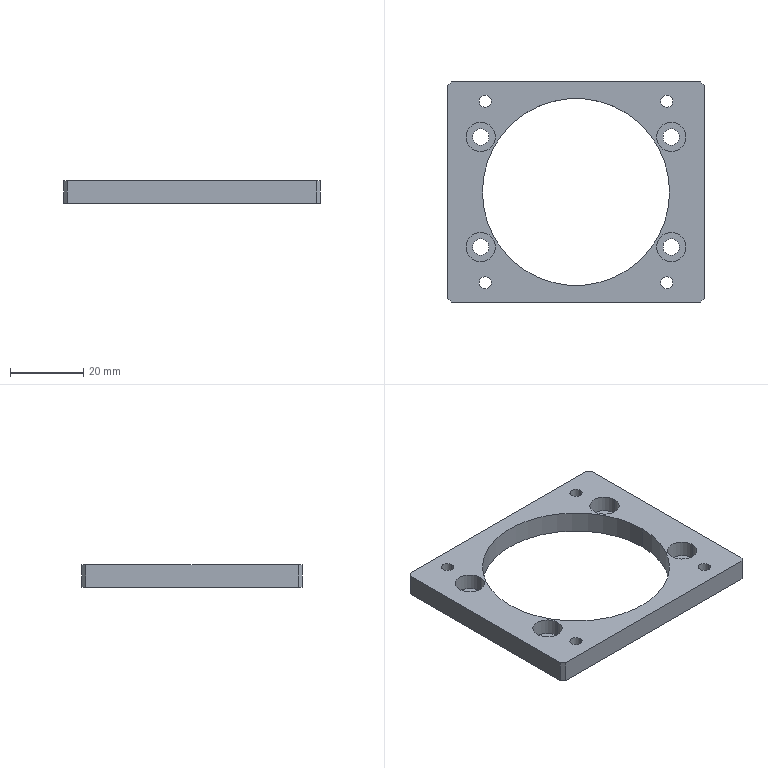Part | NX | features BREP 1 | 1 solid | 40 faces | box 70 x 60 x 6 mm | volume 11726 mm3 | cylinder 26 | plane 14 | commonest cylinder face diameters 3.3 x8 4.5 x8 8 x8 51 x2
STEP:
#1=CARTESIAN_POINT('',(58.099,54.749,0.));
#2=VERTEX_POINT('',#1);
#3=CARTESIAN_POINT('',(61.399,54.749,0.));
#4=VERTEX_POINT('',#3);
#5=CARTESIAN_POINT('',(59.749,54.749,0.));
#6=DIRECTION('',(0.,0.,1.));
#7=DIRECTION('',(1.,0.,0.));
#8=AXIS2_PLACEMENT_3D('',#5,#6,#7);
#9=CIRCLE('',#8,1.65);
#10=EDGE_CURVE('',#2,#4,#9,.T.);
#11=ORIENTED_EDGE('',*,*,#10,.F.);
#12=CARTESIAN_POINT('',(58.099,54.749,6.));
#13=VERTEX_POINT('',#12);
#14=CARTESIAN_POINT('',(58.099,54.749,6.));
#15=DIRECTION('',(0.,0.,1.));
#16=VECTOR('',#15,1000.);
#17=LINE('',#14,#16);
#18=EDGE_CURVE('',#13,#2,#17,.F.);
#19=ORIENTED_EDGE('',*,*,#18,.F.);
#20=CARTESIAN_POINT('',(61.399,54.749,6.));
#21=VERTEX_POINT('',#20);
#22=CARTESIAN_POINT('',(59.749,54.749,6.));
#23=DIRECTION('',(0.,0.,1.));
#24=DIRECTION('',(1.,0.,0.));
#25=AXIS2_PLACEMENT_3D('',#22,#23,#24);
#26=CIRCLE('',#25,1.65);
#27=EDGE_CURVE('',#13,#21,#26,.T.);
#28=ORIENTED_EDGE('',*,*,#27,.T.);
#29=CARTESIAN_POINT('',(61.399,54.749,6.));
#30=DIRECTION('',(0.,0.,1.));
#31=VECTOR('',#30,1000.);
#32=LINE('',#29,#31);
#33=EDGE_CURVE('',#21,#4,#32,.F.);
#34=ORIENTED_EDGE('',*,*,#33,.T.);
#35=EDGE_LOOP('',(#11,#19,#28,#34));
#36=FACE_BOUND('',#35,.T.);
#37=CARTESIAN_POINT('',(59.749,54.749,6.));
#38=DIRECTION('',(0.,0.,1.));
#39=DIRECTION('',(1.,0.,0.));
#40=AXIS2_PLACEMENT_3D('',#37,#38,#39);
#41=CYLINDRICAL_SURFACE('',#40,1.65);
#42=ADVANCED_FACE('',(#36),#41,.F.);
#43=CARTESIAN_POINT('',(58.099,5.251,0.));
#44=VERTEX_POINT('',#43);
#45=CARTESIAN_POINT('',(61.399,5.251,0.));
#46=VERTEX_POINT('',#45);
#47=CARTESIAN_POINT('',(59.749,5.251,0.));
#48=DIRECTION('',(0.,0.,1.));
#49=DIRECTION('',(1.,0.,0.));
#50=AXIS2_PLACEMENT_3D('',#47,#48,#49);
#51=CIRCLE('',#50,1.65);
#52=EDGE_CURVE('',#44,#46,#51,.T.);
#53=ORIENTED_EDGE('',*,*,#52,.F.);
#54=CARTESIAN_POINT('',(58.099,5.251,6.));
#55=VERTEX_POINT('',#54);
#56=CARTESIAN_POINT('',(58.099,5.251,6.));
#57=DIRECTION('',(0.,0.,1.));
#58=VECTOR('',#57,1000.);
#59=LINE('',#56,#58);
#60=EDGE_CURVE('',#55,#44,#59,.F.);
#61=ORIENTED_EDGE('',*,*,#60,.F.);
#62=CARTESIAN_POINT('',(61.399,5.251,6.));
#63=VERTEX_POINT('',#62);
#64=CARTESIAN_POINT('',(59.749,5.251,6.));
#65=DIRECTION('',(0.,0.,1.));
#66=DIRECTION('',(1.,0.,0.));
#67=AXIS2_PLACEMENT_3D('',#64,#65,#66);
#68=CIRCLE('',#67,1.65);
#69=EDGE_CURVE('',#55,#63,#68,.T.);
#70=ORIENTED_EDGE('',*,*,#69,.T.);
#71=CARTESIAN_POINT('',(61.399,5.251,6.));
#72=DIRECTION('',(0.,0.,1.));
#73=VECTOR('',#72,1000.);
#74=LINE('',#71,#73);
#75=EDGE_CURVE('',#63,#46,#74,.F.);
#76=ORIENTED_EDGE('',*,*,#75,.T.);
#77=EDGE_LOOP('',(#53,#61,#70,#76));
#78=FACE_BOUND('',#77,.T.);
#79=CARTESIAN_POINT('',(59.749,5.251,6.));
#80=DIRECTION('',(0.,0.,1.));
#81=DIRECTION('',(1.,0.,0.));
#82=AXIS2_PLACEMENT_3D('',#79,#80,#81);
#83=CYLINDRICAL_SURFACE('',#82,1.65);
#84=ADVANCED_FACE('',(#78),#83,.F.);
#85=CARTESIAN_POINT('',(8.601,5.251,0.));
#86=VERTEX_POINT('',#85);
#87=CARTESIAN_POINT('',(11.901,5.251,0.));
#88=VERTEX_POINT('',#87);
#89=CARTESIAN_POINT('',(10.251,5.251,0.));
#90=DIRECTION('',(0.,0.,1.));
#91=DIRECTION('',(1.,0.,0.));
#92=AXIS2_PLACEMENT_3D('',#89,#90,#91);
#93=CIRCLE('',#92,1.65);
#94=EDGE_CURVE('',#86,#88,#93,.T.);
#95=ORIENTED_EDGE('',*,*,#94,.F.);
#96=CARTESIAN_POINT('',(8.601,5.251,6.));
#97=VERTEX_POINT('',#96);
#98=CARTESIAN_POINT('',(8.601,5.251,6.));
#99=DIRECTION('',(0.,0.,1.));
#100=VECTOR('',#99,1000.);
#101=LINE('',#98,#100);
#102=EDGE_CURVE('',#97,#86,#101,.F.);
#103=ORIENTED_EDGE('',*,*,#102,.F.);
#104=CARTESIAN_POINT('',(11.901,5.251,6.));
#105=VERTEX_POINT('',#104);
#106=CARTESIAN_POINT('',(10.251,5.251,6.));
#107=DIRECTION('',(0.,0.,1.));
#108=DIRECTION('',(1.,0.,0.));
#109=AXIS2_PLACEMENT_3D('',#106,#107,#108);
#110=CIRCLE('',#109,1.65);
#111=EDGE_CURVE('',#97,#105,#110,.T.);
#112=ORIENTED_EDGE('',*,*,#111,.T.);
#113=CARTESIAN_POINT('',(11.901,5.251,6.));
#114=DIRECTION('',(0.,0.,1.));
#115=VECTOR('',#114,1000.);
#116=LINE('',#113,#115);
#117=EDGE_CURVE('',#105,#88,#116,.F.);
#118=ORIENTED_EDGE('',*,*,#117,.T.);
#119=EDGE_LOOP('',(#95,#103,#112,#118));
#120=FACE_BOUND('',#119,.T.);
#121=CARTESIAN_POINT('',(10.251,5.251,6.));
#122=DIRECTION('',(0.,0.,1.));
#123=DIRECTION('',(1.,0.,0.));
#124=AXIS2_PLACEMENT_3D('',#121,#122,#123);
#125=CYLINDRICAL_SURFACE('',#124,1.65);
#126=ADVANCED_FACE('',(#120),#125,.F.);
#127=CARTESIAN_POINT('',(8.601,54.749,0.));
#128=VERTEX_POINT('',#127);
#129=CARTESIAN_POINT('',(11.901,54.749,0.));
#130=VERTEX_POINT('',#129);
#131=CARTESIAN_POINT('',(10.251,54.749,0.));
#132=DIRECTION('',(0.,0.,1.));
#133=DIRECTION('',(1.,0.,0.));
#134=AXIS2_PLACEMENT_3D('',#131,#132,#133);
#135=CIRCLE('',#134,1.65);
#136=EDGE_CURVE('',#128,#130,#135,.T.);
#137=ORIENTED_EDGE('',*,*,#136,.F.);
#138=CARTESIAN_POINT('',(8.601,54.749,6.));
#139=VERTEX_POINT('',#138);
#140=CARTESIAN_POINT('',(8.601,54.749,6.));
#141=DIRECTION('',(0.,0.,1.));
#142=VECTOR('',#141,1000.);
#143=LINE('',#140,#142);
#144=EDGE_CURVE('',#139,#128,#143,.F.);
#145=ORIENTED_EDGE('',*,*,#144,.F.);
#146=CARTESIAN_POINT('',(11.901,54.749,6.));
#147=VERTEX_POINT('',#146);
#148=CARTESIAN_POINT('',(10.251,54.749,6.));
#149=DIRECTION('',(0.,0.,1.));
#150=DIRECTION('',(1.,0.,0.));
#151=AXIS2_PLACEMENT_3D('',#148,#149,#150);
#152=CIRCLE('',#151,1.65);
#153=EDGE_CURVE('',#139,#147,#152,.T.);
#154=ORIENTED_EDGE('',*,*,#153,.T.);
#155=CARTESIAN_POINT('',(11.901,54.749,6.));
#156=DIRECTION('',(0.,0.,1.));
#157=VECTOR('',#156,1000.);
#158=LINE('',#155,#157);
#159=EDGE_CURVE('',#147,#130,#158,.F.);
#160=ORIENTED_EDGE('',*,*,#159,.T.);
#161=EDGE_LOOP('',(#137,#145,#154,#160));
#162=FACE_BOUND('',#161,.T.);
#163=CARTESIAN_POINT('',(10.251,54.749,6.));
#164=DIRECTION('',(0.,0.,1.));
#165=DIRECTION('',(1.,0.,0.));
#166=AXIS2_PLACEMENT_3D('',#163,#164,#165);
#167=CYLINDRICAL_SURFACE('',#166,1.65);
#168=ADVANCED_FACE('',(#162),#167,.F.);
#169=CARTESIAN_POINT('',(56.981,45.,1.5));
#170=VERTEX_POINT('',#169);
#171=CARTESIAN_POINT('',(64.981,45.,1.5));
#172=VERTEX_POINT('',#171);
#173=CARTESIAN_POINT('',(60.981,45.,1.5));
#174=DIRECTION('',(0.,0.,1.));
#175=DIRECTION('',(1.,0.,0.));
#176=AXIS2_PLACEMENT_3D('',#173,#174,#175);
#177=CIRCLE('',#176,4.);
#178=EDGE_CURVE('',#170,#172,#177,.T.);
#179=ORIENTED_EDGE('',*,*,#178,.F.);
#180=CARTESIAN_POINT('',(56.981,45.,6.));
#181=VERTEX_POINT('',#180);
#182=CARTESIAN_POINT('',(56.981,45.,6.));
#183=DIRECTION('',(0.,0.,1.));
#184=VECTOR('',#183,1000.);
#185=LINE('',#182,#184);
#186=EDGE_CURVE('',#181,#170,#185,.F.);
#187=ORIENTED_EDGE('',*,*,#186,.F.);
#188=CARTESIAN_POINT('',(64.981,45.,6.));
#189=VERTEX_POINT('',#188);
#190=CARTESIAN_POINT('',(60.981,45.,6.));
#191=DIRECTION('',(0.,0.,1.));
#192=DIRECTION('',(1.,0.,0.));
#193=AXIS2_PLACEMENT_3D('',#190,#191,#192);
#194=CIRCLE('',#193,4.);
#195=EDGE_CURVE('',#181,#189,#194,.T.);
#196=ORIENTED_EDGE('',*,*,#195,.T.);
#197=CARTESIAN_POINT('',(64.981,45.,6.));
#198=DIRECTION('',(0.,0.,1.));
#199=VECTOR('',#198,1000.);
#200=LINE('',#197,#199);
#201=EDGE_CURVE('',#189,#172,#200,.F.);
#202=ORIENTED_EDGE('',*,*,#201,.T.);
#203=EDGE_LOOP('',(#179,#187,#196,#202));
#204=FACE_BOUND('',#203,.T.);
#205=CARTESIAN_POINT('',(60.981,45.,6.));
#206=DIRECTION('',(0.,0.,1.));
#207=DIRECTION('',(1.,0.,0.));
#208=AXIS2_PLACEMENT_3D('',#205,#206,#207);
#209=CYLINDRICAL_SURFACE('',#208,4.);
#210=ADVANCED_FACE('',(#204),#209,.F.);
#211=CARTESIAN_POINT('',(58.731,45.,0.));
#212=VERTEX_POINT('',#211);
#213=CARTESIAN_POINT('',(63.231,45.,0.));
#214=VERTEX_POINT('',#213);
#215=CARTESIAN_POINT('',(60.981,45.,0.));
#216=DIRECTION('',(0.,0.,1.));
#217=DIRECTION('',(1.,0.,0.));
#218=AXIS2_PLACEMENT_3D('',#215,#216,#217);
#219=CIRCLE('',#218,2.25);
#220=EDGE_CURVE('',#212,#214,#219,.T.);
#221=ORIENTED_EDGE('',*,*,#220,.F.);
#222=CARTESIAN_POINT('',(58.731,45.,1.5));
#223=VERTEX_POINT('',#222);
#224=CARTESIAN_POINT('',(58.731,45.,6.));
#225=DIRECTION('',(0.,0.,1.));
#226=VECTOR('',#225,1000.);
#227=LINE('',#224,#226);
#228=EDGE_CURVE('',#223,#212,#227,.F.);
#229=ORIENTED_EDGE('',*,*,#228,.F.);
#230=CARTESIAN_POINT('',(63.231,45.,1.5));
#231=VERTEX_POINT('',#230);
#232=CARTESIAN_POINT('',(60.981,45.,1.5));
#233=DIRECTION('',(0.,0.,1.));
#234=DIRECTION('',(1.,0.,0.));
#235=AXIS2_PLACEMENT_3D('',#232,#233,#234);
#236=CIRCLE('',#235,2.25);
#237=EDGE_CURVE('',#223,#231,#236,.T.);
#238=ORIENTED_EDGE('',*,*,#237,.T.);
#239=CARTESIAN_POINT('',(63.231,45.,6.));
#240=DIRECTION('',(0.,0.,1.));
#241=VECTOR('',#240,1000.);
#242=LINE('',#239,#241);
#243=EDGE_CURVE('',#231,#214,#242,.F.);
#244=ORIENTED_EDGE('',*,*,#243,.T.);
#245=EDGE_LOOP('',(#221,#229,#238,#244));
#246=FACE_BOUND('',#245,.T.);
#247=CARTESIAN_POINT('',(60.981,45.,6.));
#248=DIRECTION('',(0.,0.,1.));
#249=DIRECTION('',(1.,0.,0.));
#250=AXIS2_PLACEMENT_3D('',#247,#248,#249);
#251=CYLINDRICAL_SURFACE('',#250,2.25);
#252=ADVANCED_FACE('',(#246),#251,.F.);
#253=CARTESIAN_POINT('',(5.019,15.,1.5));
#254=VERTEX_POINT('',#253);
#255=CARTESIAN_POINT('',(13.019,15.,1.5));
#256=VERTEX_POINT('',#255);
#257=CARTESIAN_POINT('',(9.019,15.,1.5));
#258=DIRECTION('',(0.,0.,1.));
#259=DIRECTION('',(1.,0.,0.));
#260=AXIS2_PLACEMENT_3D('',#257,#258,#259);
#261=CIRCLE('',#260,4.);
#262=EDGE_CURVE('',#254,#256,#261,.T.);
#263=ORIENTED_EDGE('',*,*,#262,.F.);
#264=CARTESIAN_POINT('',(5.019,15.,6.));
#265=VERTEX_POINT('',#264);
#266=CARTESIAN_POINT('',(5.019,15.,6.));
#267=DIRECTION('',(0.,0.,1.));
#268=VECTOR('',#267,1000.);
#269=LINE('',#266,#268);
#270=EDGE_CURVE('',#265,#254,#269,.F.);
#271=ORIENTED_EDGE('',*,*,#270,.F.);
#272=CARTESIAN_POINT('',(13.019,15.,6.));
#273=VERTEX_POINT('',#272);
#274=CARTESIAN_POINT('',(9.019,15.,6.));
#275=DIRECTION('',(0.,0.,1.));
#276=DIRECTION('',(1.,0.,0.));
#277=AXIS2_PLACEMENT_3D('',#274,#275,#276);
#278=CIRCLE('',#277,4.);
#279=EDGE_CURVE('',#265,#273,#278,.T.);
#280=ORIENTED_EDGE('',*,*,#279,.T.);
#281=CARTESIAN_POINT('',(13.019,15.,6.));
#282=DIRECTION('',(0.,0.,1.));
#283=VECTOR('',#282,1000.);
#284=LINE('',#281,#283);
#285=EDGE_CURVE('',#273,#256,#284,.F.);
#286=ORIENTED_EDGE('',*,*,#285,.T.);
#287=EDGE_LOOP('',(#263,#271,#280,#286));
#288=FACE_BOUND('',#287,.T.);
#289=CARTESIAN_POINT('',(9.019,15.,6.));
#290=DIRECTION('',(0.,0.,1.));
#291=DIRECTION('',(1.,0.,0.));
#292=AXIS2_PLACEMENT_3D('',#289,#290,#291);
#293=CYLINDRICAL_SURFACE('',#292,4.);
#294=ADVANCED_FACE('',(#288),#293,.F.);
#295=CARTESIAN_POINT('',(6.769,15.,0.));
#296=VERTEX_POINT('',#295);
#297=CARTESIAN_POINT('',(11.269,15.,0.));
#298=VERTEX_POINT('',#297);
#299=CARTESIAN_POINT('',(9.019,15.,0.));
#300=DIRECTION('',(0.,0.,1.));
#301=DIRECTION('',(1.,0.,0.));
#302=AXIS2_PLACEMENT_3D('',#299,#300,#301);
#303=CIRCLE('',#302,2.25);
#304=EDGE_CURVE('',#296,#298,#303,.T.);
#305=ORIENTED_EDGE('',*,*,#304,.F.);
#306=CARTESIAN_POINT('',(6.769,15.,1.5));
#307=VERTEX_POINT('',#306);
#308=CARTESIAN_POINT('',(6.769,15.,6.));
#309=DIRECTION('',(0.,0.,1.));
#310=VECTOR('',#309,1000.);
#311=LINE('',#308,#310);
#312=EDGE_CURVE('',#307,#296,#311,.F.);
#313=ORIENTED_EDGE('',*,*,#312,.F.);
#314=CARTESIAN_POINT('',(11.269,15.,1.5));
#315=VERTEX_POINT('',#314);
#316=CARTESIAN_POINT('',(9.019,15.,1.5));
#317=DIRECTION('',(0.,0.,1.));
#318=DIRECTION('',(1.,0.,0.));
#319=AXIS2_PLACEMENT_3D('',#316,#317,#318);
#320=CIRCLE('',#319,2.25);
#321=EDGE_CURVE('',#307,#315,#320,.T.);
#322=ORIENTED_EDGE('',*,*,#321,.T.);
#323=CARTESIAN_POINT('',(11.269,15.,6.));
#324=DIRECTION('',(0.,0.,1.));
#325=VECTOR('',#324,1000.);
#326=LINE('',#323,#325);
#327=EDGE_CURVE('',#315,#298,#326,.F.);
#328=ORIENTED_EDGE('',*,*,#327,.T.);
#329=EDGE_LOOP('',(#305,#313,#322,#328));
#330=FACE_BOUND('',#329,.T.);
#331=CARTESIAN_POINT('',(9.019,15.,6.));
#332=DIRECTION('',(0.,0.,1.));
#333=DIRECTION('',(1.,0.,0.));
#334=AXIS2_PLACEMENT_3D('',#331,#332,#333);
#335=CYLINDRICAL_SURFACE('',#334,2.25);
#336=ADVANCED_FACE('',(#330),#335,.F.);
#337=CARTESIAN_POINT('',(5.019,45.,1.5));
#338=VERTEX_POINT('',#337);
#339=CARTESIAN_POINT('',(13.019,45.,1.5));
#340=VERTEX_POINT('',#339);
#341=CARTESIAN_POINT('',(9.019,45.,1.5));
#342=DIRECTION('',(0.,0.,1.));
#343=DIRECTION('',(1.,0.,0.));
#344=AXIS2_PLACEMENT_3D('',#341,#342,#343);
#345=CIRCLE('',#344,4.);
#346=EDGE_CURVE('',#338,#340,#345,.T.);
#347=ORIENTED_EDGE('',*,*,#346,.F.);
#348=CARTESIAN_POINT('',(5.019,45.,6.));
#349=VERTEX_POINT('',#348);
#350=CARTESIAN_POINT('',(5.019,45.,6.));
#351=DIRECTION('',(0.,0.,1.));
#352=VECTOR('',#351,1000.);
#353=LINE('',#350,#352);
#354=EDGE_CURVE('',#349,#338,#353,.F.);
#355=ORIENTED_EDGE('',*,*,#354,.F.);
#356=CARTESIAN_POINT('',(13.019,45.,6.));
#357=VERTEX_POINT('',#356);
#358=CARTESIAN_POINT('',(9.019,45.,6.));
#359=DIRECTION('',(0.,0.,1.));
#360=DIRECTION('',(1.,0.,0.));
#361=AXIS2_PLACEMENT_3D('',#358,#359,#360);
#362=CIRCLE('',#361,4.);
#363=EDGE_CURVE('',#349,#357,#362,.T.);
#364=ORIENTED_EDGE('',*,*,#363,.T.);
#365=CARTESIAN_POINT('',(13.019,45.,6.));
#366=DIRECTION('',(0.,0.,1.));
#367=VECTOR('',#366,1000.);
#368=LINE('',#365,#367);
#369=EDGE_CURVE('',#357,#340,#368,.F.);
#370=ORIENTED_EDGE('',*,*,#369,.T.);
#371=EDGE_LOOP('',(#347,#355,#364,#370));
#372=FACE_BOUND('',#371,.T.);
#373=CARTESIAN_POINT('',(9.019,45.,6.));
#374=DIRECTION('',(0.,0.,1.));
#375=DIRECTION('',(1.,0.,0.));
#376=AXIS2_PLACEMENT_3D('',#373,#374,#375);
#377=CYLINDRICAL_SURFACE('',#376,4.);
#378=ADVANCED_FACE('',(#372),#377,.F.);
#379=CARTESIAN_POINT('',(6.769,45.,0.));
#380=VERTEX_POINT('',#379);
#381=CARTESIAN_POINT('',(11.269,45.,0.));
#382=VERTEX_POINT('',#381);
#383=CARTESIAN_POINT('',(9.019,45.,0.));
#384=DIRECTION('',(0.,0.,1.));
#385=DIRECTION('',(1.,0.,0.));
#386=AXIS2_PLACEMENT_3D('',#383,#384,#385);
#387=CIRCLE('',#386,2.25);
#388=EDGE_CURVE('',#380,#382,#387,.T.);
#389=ORIENTED_EDGE('',*,*,#388,.F.);
#390=CARTESIAN_POINT('',(6.769,45.,1.5));
#391=VERTEX_POINT('',#390);
#392=CARTESIAN_POINT('',(6.769,45.,6.));
#393=DIRECTION('',(0.,0.,1.));
#394=VECTOR('',#393,1000.);
#395=LINE('',#392,#394);
#396=EDGE_CURVE('',#391,#380,#395,.F.);
#397=ORIENTED_EDGE('',*,*,#396,.F.);
#398=CARTESIAN_POINT('',(11.269,45.,1.5));
#399=VERTEX_POINT('',#398);
#400=CARTESIAN_POINT('',(9.019,45.,1.5));
#401=DIRECTION('',(0.,0.,1.));
#402=DIRECTION('',(1.,0.,0.));
#403=AXIS2_PLACEMENT_3D('',#400,#401,#402);
#404=CIRCLE('',#403,2.25);
#405=EDGE_CURVE('',#391,#399,#404,.T.);
#406=ORIENTED_EDGE('',*,*,#405,.T.);
#407=CARTESIAN_POINT('',(11.269,45.,6.));
#408=DIRECTION('',(0.,0.,1.));
#409=VECTOR('',#408,1000.);
#410=LINE('',#407,#409);
#411=EDGE_CURVE('',#399,#382,#410,.F.);
#412=ORIENTED_EDGE('',*,*,#411,.T.);
#413=EDGE_LOOP('',(#389,#397,#406,#412));
#414=FACE_BOUND('',#413,.T.);
#415=CARTESIAN_POINT('',(9.019,45.,6.));
#416=DIRECTION('',(0.,0.,1.));
#417=DIRECTION('',(1.,0.,0.));
#418=AXIS2_PLACEMENT_3D('',#415,#416,#417);
#419=CYLINDRICAL_SURFACE('',#418,2.25);
#420=ADVANCED_FACE('',(#414),#419,.F.);
#421=CARTESIAN_POINT('',(56.981,15.,1.5));
#422=VERTEX_POINT('',#421);
#423=CARTESIAN_POINT('',(64.981,15.,1.5));
#424=VERTEX_POINT('',#423);
#425=CARTESIAN_POINT('',(60.981,15.,1.5));
#426=DIRECTION('',(0.,0.,1.));
#427=DIRECTION('',(1.,0.,0.));
#428=AXIS2_PLACEMENT_3D('',#425,#426,#427);
#429=CIRCLE('',#428,4.);
#430=EDGE_CURVE('',#422,#424,#429,.T.);
#431=ORIENTED_EDGE('',*,*,#430,.F.);
#432=CARTESIAN_POINT('',(56.981,15.,6.));
#433=VERTEX_POINT('',#432);
#434=CARTESIAN_POINT('',(56.981,15.,6.));
#435=DIRECTION('',(0.,0.,1.));
#436=VECTOR('',#435,1000.);
#437=LINE('',#434,#436);
#438=EDGE_CURVE('',#433,#422,#437,.F.);
#439=ORIENTED_EDGE('',*,*,#438,.F.);
#440=CARTESIAN_POINT('',(64.981,15.,6.));
#441=VERTEX_POINT('',#440);
#442=CARTESIAN_POINT('',(60.981,15.,6.));
#443=DIRECTION('',(0.,0.,1.));
#444=DIRECTION('',(1.,0.,0.));
#445=AXIS2_PLACEMENT_3D('',#442,#443,#444);
#446=CIRCLE('',#445,4.);
#447=EDGE_CURVE('',#433,#441,#446,.T.);
#448=ORIENTED_EDGE('',*,*,#447,.T.);
#449=CARTESIAN_POINT('',(64.981,15.,6.));
#450=DIRECTION('',(0.,0.,1.));
#451=VECTOR('',#450,1000.);
#452=LINE('',#449,#451);
#453=EDGE_CURVE('',#441,#424,#452,.F.);
#454=ORIENTED_EDGE('',*,*,#453,.T.);
#455=EDGE_LOOP('',(#431,#439,#448,#454));
#456=FACE_BOUND('',#455,.T.);
#457=CARTESIAN_POINT('',(60.981,15.,6.));
#458=DIRECTION('',(0.,0.,1.));
#459=DIRECTION('',(1.,0.,0.));
#460=AXIS2_PLACEMENT_3D('',#457,#458,#459);
#461=CYLINDRICAL_SURFACE('',#460,4.);
#462=ADVANCED_FACE('',(#456),#461,.F.);
#463=CARTESIAN_POINT('',(58.731,15.,0.));
#464=VERTEX_POINT('',#463);
#465=CARTESIAN_POINT('',(63.231,15.,0.));
#466=VERTEX_POINT('',#465);
#467=CARTESIAN_POINT('',(60.981,15.,0.));
#468=DIRECTION('',(0.,0.,1.));
#469=DIRECTION('',(1.,0.,0.));
#470=AXIS2_PLACEMENT_3D('',#467,#468,#469);
#471=CIRCLE('',#470,2.25);
#472=EDGE_CURVE('',#464,#466,#471,.T.);
#473=ORIENTED_EDGE('',*,*,#472,.F.);
#474=CARTESIAN_POINT('',(58.731,15.,1.5));
#475=VERTEX_POINT('',#474);
#476=CARTESIAN_POINT('',(58.731,15.,6.));
#477=DIRECTION('',(0.,0.,1.));
#478=VECTOR('',#477,1000.);
#479=LINE('',#476,#478);
#480=EDGE_CURVE('',#475,#464,#479,.F.);
#481=ORIENTED_EDGE('',*,*,#480,.F.);
#482=CARTESIAN_POINT('',(63.231,15.,1.5));
#483=VERTEX_POINT('',#482);
#484=CARTESIAN_POINT('',(60.981,15.,1.5));
#485=DIRECTION('',(0.,0.,1.));
#486=DIRECTION('',(1.,0.,0.));
#487=AXIS2_PLACEMENT_3D('',#484,#485,#486);
#488=CIRCLE('',#487,2.25);
#489=EDGE_CURVE('',#475,#483,#488,.T.);
#490=ORIENTED_EDGE('',*,*,#489,.T.);
#491=CARTESIAN_POINT('',(63.231,15.,6.));
#492=DIRECTION('',(0.,0.,1.));
#493=VECTOR('',#492,1000.);
#494=LINE('',#491,#493);
#495=EDGE_CURVE('',#483,#466,#494,.F.);
#496=ORIENTED_EDGE('',*,*,#495,.T.);
#497=EDGE_LOOP('',(#473,#481,#490,#496));
#498=FACE_BOUND('',#497,.T.);
#499=CARTESIAN_POINT('',(60.981,15.,6.));
#500=DIRECTION('',(0.,0.,1.));
#501=DIRECTION('',(1.,0.,0.));
#502=AXIS2_PLACEMENT_3D('',#499,#500,#501);
#503=CYLINDRICAL_SURFACE('',#502,2.25);
#504=ADVANCED_FACE('',(#498),#503,.F.);
#505=CARTESIAN_POINT('',(60.5,30.,0.));
#506=VERTEX_POINT('',#505);
#507=CARTESIAN_POINT('',(9.5,30.,0.));
#508=VERTEX_POINT('',#507);
#509=CARTESIAN_POINT('',(35.,30.,0.));
#510=DIRECTION('',(0.,0.,-1.));
#511=DIRECTION('',(-1.,0.,0.));
#512=AXIS2_PLACEMENT_3D('',#509,#510,#511);
#513=CIRCLE('',#512,25.5);
#514=EDGE_CURVE('',#506,#508,#513,.T.);
#515=ORIENTED_EDGE('',*,*,#514,.T.);
#516=CARTESIAN_POINT('',(9.5,30.,6.));
#517=VERTEX_POINT('',#516);
#518=CARTESIAN_POINT('',(9.5,30.,-4.));
#519=DIRECTION('',(0.,0.,1.));
#520=VECTOR('',#519,1000.);
#521=LINE('',#518,#520);
#522=EDGE_CURVE('',#517,#508,#521,.F.);
#523=ORIENTED_EDGE('',*,*,#522,.F.);
#524=CARTESIAN_POINT('',(60.5,30.,6.));
#525=VERTEX_POINT('',#524);
#526=CARTESIAN_POINT('',(35.,30.,6.));
#527=DIRECTION('',(0.,0.,1.));
#528=DIRECTION('',(1.,0.,0.));
#529=AXIS2_PLACEMENT_3D('',#526,#527,#528);
#530=CIRCLE('',#529,25.5);
#531=EDGE_CURVE('',#517,#525,#530,.T.);
#532=ORIENTED_EDGE('',*,*,#531,.T.);
#533=CARTESIAN_POINT('',(60.5,30.,-4.));
#534=DIRECTION('',(0.,0.,1.));
#535=VECTOR('',#534,1000.);
#536=LINE('',#533,#535);
#537=EDGE_CURVE('',#525,#506,#536,.F.);
#538=ORIENTED_EDGE('',*,*,#537,.T.);
#539=EDGE_LOOP('',(#515,#523,#532,#538));
#540=FACE_BOUND('',#539,.T.);
#541=CARTESIAN_POINT('',(35.,30.,-4.));
#542=DIRECTION('',(0.,0.,1.));
#543=DIRECTION('',(1.,0.,0.));
#544=AXIS2_PLACEMENT_3D('',#541,#542,#543);
#545=CYLINDRICAL_SURFACE('',#544,25.5);
#546=ADVANCED_FACE('',(#540),#545,.F.);
#547=CARTESIAN_POINT('',(1.,0.,0.));
#548=VERTEX_POINT('',#547);
#549=CARTESIAN_POINT('',(69.,0.,0.));
#550=VERTEX_POINT('',#549);
#551=CARTESIAN_POINT('',(0.,0.,0.));
#552=DIRECTION('',(1.,0.,0.));
#553=VECTOR('',#552,1000.);
#554=LINE('',#551,#553);
#555=EDGE_CURVE('',#548,#550,#554,.T.);
#556=ORIENTED_EDGE('',*,*,#555,.F.);
#557=CARTESIAN_POINT('',(0.,1.,0.));
#558=VERTEX_POINT('',#557);
#559=CARTESIAN_POINT('',(0.5,0.5,0.));
#560=DIRECTION('',(-0.7071,0.7071,0.));
#561=VECTOR('',#560,1000.);
#562=LINE('',#559,#561);
#563=EDGE_CURVE('',#548,#558,#562,.T.);
#564=ORIENTED_EDGE('',*,*,#563,.T.);
#565=CARTESIAN_POINT('',(0.,59.,0.));
#566=VERTEX_POINT('',#565);
#567=CARTESIAN_POINT('',(0.,0.,0.));
#568=DIRECTION('',(0.,-1.,0.));
#569=VECTOR('',#568,1000.);
#570=LINE('',#567,#569);
#571=EDGE_CURVE('',#566,#558,#570,.T.);
#572=ORIENTED_EDGE('',*,*,#571,.F.);
#573=CARTESIAN_POINT('',(1.,60.,0.));
#574=VERTEX_POINT('',#573);
#575=CARTESIAN_POINT('',(-29.5,29.5,0.));
#576=DIRECTION('',(0.7071,0.7071,0.));
#577=VECTOR('',#576,1000.);
#578=LINE('',#575,#577);
#579=EDGE_CURVE('',#566,#574,#578,.T.);
#580=ORIENTED_EDGE('',*,*,#579,.T.);
#581=CARTESIAN_POINT('',(69.,60.,0.));
#582=VERTEX_POINT('',#581);
#583=CARTESIAN_POINT('',(0.,60.,0.));
#584=DIRECTION('',(-1.,0.,0.));
#585=VECTOR('',#584,1000.);
#586=LINE('',#583,#585);
#587=EDGE_CURVE('',#582,#574,#586,.T.);
#588=ORIENTED_EDGE('',*,*,#587,.F.);
#589=CARTESIAN_POINT('',(70.,59.,0.));
#590=VERTEX_POINT('',#589);
#591=CARTESIAN_POINT('',(64.5,64.5,0.));
#592=DIRECTION('',(0.7071,-0.7071,0.));
#593=VECTOR('',#592,1000.);
#594=LINE('',#591,#593);
#595=EDGE_CURVE('',#582,#590,#594,.T.);
#596=ORIENTED_EDGE('',*,*,#595,.T.);
#597=CARTESIAN_POINT('',(70.,1.,0.));
#598=VERTEX_POINT('',#597);
#599=CARTESIAN_POINT('',(70.,0.,0.));
#600=DIRECTION('',(0.,1.,0.));
#601=VECTOR('',#600,1000.);
#602=LINE('',#599,#601);
#603=EDGE_CURVE('',#598,#590,#602,.T.);
#604=ORIENTED_EDGE('',*,*,#603,.F.);
#605=CARTESIAN_POINT('',(34.5,-34.5,0.));
#606=DIRECTION('',(-0.7071,-0.7071,0.));
#607=VECTOR('',#606,1000.);
#608=LINE('',#605,#607);
#609=EDGE_CURVE('',#598,#550,#608,.T.);
#610=ORIENTED_EDGE('',*,*,#609,.T.);
#611=EDGE_LOOP('',(#556,#564,#572,#580,#588,#596,#604,#610));
#612=FACE_BOUND('',#611,.T.);
#613=CARTESIAN_POINT('',(59.749,54.749,0.));
#614=DIRECTION('',(0.,0.,1.));
#615=DIRECTION('',(1.,0.,0.));
#616=AXIS2_PLACEMENT_3D('',#613,#614,#615);
#617=CIRCLE('',#616,1.65);
#618=EDGE_CURVE('',#4,#2,#617,.T.);
#619=ORIENTED_EDGE('',*,*,#618,.T.);
#620=ORIENTED_EDGE('',*,*,#10,.T.);
#621=EDGE_LOOP('',(#619,#620));
#622=FACE_BOUND('',#621,.T.);
#623=CARTESIAN_POINT('',(59.749,5.251,0.));
#624=DIRECTION('',(0.,0.,1.));
#625=DIRECTION('',(1.,0.,0.));
#626=AXIS2_PLACEMENT_3D('',#623,#624,#625);
#627=CIRCLE('',#626,1.65);
#628=EDGE_CURVE('',#46,#44,#627,.T.);
#629=ORIENTED_EDGE('',*,*,#628,.T.);
#630=ORIENTED_EDGE('',*,*,#52,.T.);
#631=EDGE_LOOP('',(#629,#630));
#632=FACE_BOUND('',#631,.T.);
#633=CARTESIAN_POINT('',(10.251,5.251,0.));
#634=DIRECTION('',(0.,0.,1.));
#635=DIRECTION('',(1.,0.,0.));
#636=AXIS2_PLACEMENT_3D('',#633,#634,#635);
#637=CIRCLE('',#636,1.65);
#638=EDGE_CURVE('',#88,#86,#637,.T.);
#639=ORIENTED_EDGE('',*,*,#638,.T.);
#640=ORIENTED_EDGE('',*,*,#94,.T.);
#641=EDGE_LOOP('',(#639,#640));
#642=FACE_BOUND('',#641,.T.);
#643=ORIENTED_EDGE('',*,*,#514,.F.);
#644=CARTESIAN_POINT('',(35.,30.,0.));
#645=DIRECTION('',(0.,0.,-1.));
#646=DIRECTION('',(-1.,0.,0.));
#647=AXIS2_PLACEMENT_3D('',#644,#645,#646);
#648=CIRCLE('',#647,25.5);
#649=EDGE_CURVE('',#508,#506,#648,.T.);
#650=ORIENTED_EDGE('',*,*,#649,.F.);
#651=EDGE_LOOP('',(#643,#650));
#652=FACE_BOUND('',#651,.T.);
#653=CARTESIAN_POINT('',(60.981,15.,0.));
#654=DIRECTION('',(0.,0.,1.));
#655=DIRECTION('',(1.,0.,0.));
#656=AXIS2_PLACEMENT_3D('',#653,#654,#655);
#657=CIRCLE('',#656,2.25);
#658=EDGE_CURVE('',#466,#464,#657,.T.);
#659=ORIENTED_EDGE('',*,*,#658,.T.);
#660=ORIENTED_EDGE('',*,*,#472,.T.);
#661=EDGE_LOOP('',(#659,#660));
#662=FACE_BOUND('',#661,.T.);
#663=CARTESIAN_POINT('',(9.019,45.,0.));
#664=DIRECTION('',(0.,0.,1.));
#665=DIRECTION('',(1.,0.,0.));
#666=AXIS2_PLACEMENT_3D('',#663,#664,#665);
#667=CIRCLE('',#666,2.25);
#668=EDGE_CURVE('',#382,#380,#667,.T.);
#669=ORIENTED_EDGE('',*,*,#668,.T.);
#670=ORIENTED_EDGE('',*,*,#388,.T.);
#671=EDGE_LOOP('',(#669,#670));
#672=FACE_BOUND('',#671,.T.);
#673=CARTESIAN_POINT('',(9.019,15.,0.));
#674=DIRECTION('',(0.,0.,1.));
#675=DIRECTION('',(1.,0.,0.));
#676=AXIS2_PLACEMENT_3D('',#673,#674,#675);
#677=CIRCLE('',#676,2.25);
#678=EDGE_CURVE('',#298,#296,#677,.T.);
#679=ORIENTED_EDGE('',*,*,#678,.T.);
#680=ORIENTED_EDGE('',*,*,#304,.T.);
#681=EDGE_LOOP('',(#679,#680));
#682=FACE_BOUND('',#681,.T.);
#683=CARTESIAN_POINT('',(60.981,45.,0.));
#684=DIRECTION('',(0.,0.,1.));
#685=DIRECTION('',(1.,0.,0.));
#686=AXIS2_PLACEMENT_3D('',#683,#684,#685);
#687=CIRCLE('',#686,2.25);
#688=EDGE_CURVE('',#214,#212,#687,.T.);
#689=ORIENTED_EDGE('',*,*,#688,.T.);
#690=ORIENTED_EDGE('',*,*,#220,.T.);
#691=EDGE_LOOP('',(#689,#690));
#692=FACE_BOUND('',#691,.T.);
#693=CARTESIAN_POINT('',(10.251,54.749,0.));
#694=DIRECTION('',(0.,0.,1.));
#695=DIRECTION('',(1.,0.,0.));
#696=AXIS2_PLACEMENT_3D('',#693,#694,#695);
#697=CIRCLE('',#696,1.65);
#698=EDGE_CURVE('',#130,#128,#697,.T.);
#699=ORIENTED_EDGE('',*,*,#698,.T.);
#700=ORIENTED_EDGE('',*,*,#136,.T.);
#701=EDGE_LOOP('',(#699,#700));
#702=FACE_BOUND('',#701,.T.);
#703=CARTESIAN_POINT('',(0.,0.,0.));
#704=DIRECTION('',(0.,0.,-1.));
#705=DIRECTION('',(0.,-1.,0.));
#706=AXIS2_PLACEMENT_3D('',#703,#704,#705);
#707=PLANE('',#706);
#708=ADVANCED_FACE('',(#612,#622,#632,#642,#652,#662,#672,#682,#692,#702),#707,.T.);
#709=CARTESIAN_POINT('',(0.,59.,6.));
#710=VERTEX_POINT('',#709);
#711=CARTESIAN_POINT('',(0.,1.,6.));
#712=VERTEX_POINT('',#711);
#713=CARTESIAN_POINT('',(0.,0.,6.));
#714=DIRECTION('',(0.,-1.,0.));
#715=VECTOR('',#714,1000.);
#716=LINE('',#713,#715);
#717=EDGE_CURVE('',#710,#712,#716,.T.);
#718=ORIENTED_EDGE('',*,*,#717,.T.);
#719=CARTESIAN_POINT('',(1.,0.,6.));
#720=VERTEX_POINT('',#719);
#721=CARTESIAN_POINT('',(1.,0.,6.));
#722=DIRECTION('',(0.7071,-0.7071,0.));
#723=VECTOR('',#722,1000.);
#724=LINE('',#721,#723);
#725=EDGE_CURVE('',#712,#720,#724,.T.);
#726=ORIENTED_EDGE('',*,*,#725,.T.);
#727=CARTESIAN_POINT('',(69.,0.,6.));
#728=VERTEX_POINT('',#727);
#729=CARTESIAN_POINT('',(0.,0.,6.));
#730=DIRECTION('',(1.,0.,0.));
#731=VECTOR('',#730,1000.);
#732=LINE('',#729,#731);
#733=EDGE_CURVE('',#720,#728,#732,.T.);
#734=ORIENTED_EDGE('',*,*,#733,.T.);
#735=CARTESIAN_POINT('',(70.,1.,6.));
#736=VERTEX_POINT('',#735);
#737=CARTESIAN_POINT('',(70.,1.,6.));
#738=DIRECTION('',(0.7071,0.7071,0.));
#739=VECTOR('',#738,1000.);
#740=LINE('',#737,#739);
#741=EDGE_CURVE('',#728,#736,#740,.T.);
#742=ORIENTED_EDGE('',*,*,#741,.T.);
#743=CARTESIAN_POINT('',(70.,59.,6.));
#744=VERTEX_POINT('',#743);
#745=CARTESIAN_POINT('',(70.,0.,6.));
#746=DIRECTION('',(0.,1.,0.));
#747=VECTOR('',#746,1000.);
#748=LINE('',#745,#747);
#749=EDGE_CURVE('',#736,#744,#748,.T.);
#750=ORIENTED_EDGE('',*,*,#749,.T.);
#751=CARTESIAN_POINT('',(69.,60.,6.));
#752=VERTEX_POINT('',#751);
#753=CARTESIAN_POINT('',(69.,60.,6.));
#754=DIRECTION('',(-0.7071,0.7071,0.));
#755=VECTOR('',#754,1000.);
#756=LINE('',#753,#755);
#757=EDGE_CURVE('',#744,#752,#756,.T.);
#758=ORIENTED_EDGE('',*,*,#757,.T.);
#759=CARTESIAN_POINT('',(1.,60.,6.));
#760=VERTEX_POINT('',#759);
#761=CARTESIAN_POINT('',(0.,60.,6.));
#762=DIRECTION('',(-1.,0.,0.));
#763=VECTOR('',#762,1000.);
#764=LINE('',#761,#763);
#765=EDGE_CURVE('',#752,#760,#764,.T.);
#766=ORIENTED_EDGE('',*,*,#765,.T.);
#767=CARTESIAN_POINT('',(0.,59.,6.));
#768=DIRECTION('',(-0.7071,-0.7071,0.));
#769=VECTOR('',#768,1000.);
#770=LINE('',#767,#769);
#771=EDGE_CURVE('',#760,#710,#770,.T.);
#772=ORIENTED_EDGE('',*,*,#771,.T.);
#773=EDGE_LOOP('',(#718,#726,#734,#742,#750,#758,#766,#772));
#774=FACE_BOUND('',#773,.T.);
#775=CARTESIAN_POINT('',(59.749,54.749,6.));
#776=DIRECTION('',(0.,0.,1.));
#777=DIRECTION('',(1.,0.,0.));
#778=AXIS2_PLACEMENT_3D('',#775,#776,#777);
#779=CIRCLE('',#778,1.65);
#780=EDGE_CURVE('',#21,#13,#779,.T.);
#781=ORIENTED_EDGE('',*,*,#780,.F.);
#782=ORIENTED_EDGE('',*,*,#27,.F.);
#783=EDGE_LOOP('',(#781,#782));
#784=FACE_BOUND('',#783,.T.);
#785=CARTESIAN_POINT('',(59.749,5.251,6.));
#786=DIRECTION('',(0.,0.,1.));
#787=DIRECTION('',(1.,0.,0.));
#788=AXIS2_PLACEMENT_3D('',#785,#786,#787);
#789=CIRCLE('',#788,1.65);
#790=EDGE_CURVE('',#63,#55,#789,.T.);
#791=ORIENTED_EDGE('',*,*,#790,.F.);
#792=ORIENTED_EDGE('',*,*,#69,.F.);
#793=EDGE_LOOP('',(#791,#792));
#794=FACE_BOUND('',#793,.T.);
#795=CARTESIAN_POINT('',(10.251,5.251,6.));
#796=DIRECTION('',(0.,0.,1.));
#797=DIRECTION('',(1.,0.,0.));
#798=AXIS2_PLACEMENT_3D('',#795,#796,#797);
#799=CIRCLE('',#798,1.65);
#800=EDGE_CURVE('',#105,#97,#799,.T.);
#801=ORIENTED_EDGE('',*,*,#800,.F.);
#802=ORIENTED_EDGE('',*,*,#111,.F.);
#803=EDGE_LOOP('',(#801,#802));
#804=FACE_BOUND('',#803,.T.);
#805=CARTESIAN_POINT('',(10.251,54.749,6.));
#806=DIRECTION('',(0.,0.,1.));
#807=DIRECTION('',(1.,0.,0.));
#808=AXIS2_PLACEMENT_3D('',#805,#806,#807);
#809=CIRCLE('',#808,1.65);
#810=EDGE_CURVE('',#147,#139,#809,.T.);
#811=ORIENTED_EDGE('',*,*,#810,.F.);
#812=ORIENTED_EDGE('',*,*,#153,.F.);
#813=EDGE_LOOP('',(#811,#812));
#814=FACE_BOUND('',#813,.T.);
#815=CARTESIAN_POINT('',(60.981,45.,6.));
#816=DIRECTION('',(0.,0.,1.));
#817=DIRECTION('',(1.,0.,0.));
#818=AXIS2_PLACEMENT_3D('',#815,#816,#817);
#819=CIRCLE('',#818,4.);
#820=EDGE_CURVE('',#189,#181,#819,.T.);
#821=ORIENTED_EDGE('',*,*,#820,.F.);
#822=ORIENTED_EDGE('',*,*,#195,.F.);
#823=EDGE_LOOP('',(#821,#822));
#824=FACE_BOUND('',#823,.T.);
#825=CARTESIAN_POINT('',(9.019,15.,6.));
#826=DIRECTION('',(0.,0.,1.));
#827=DIRECTION('',(1.,0.,0.));
#828=AXIS2_PLACEMENT_3D('',#825,#826,#827);
#829=CIRCLE('',#828,4.);
#830=EDGE_CURVE('',#273,#265,#829,.T.);
#831=ORIENTED_EDGE('',*,*,#830,.F.);
#832=ORIENTED_EDGE('',*,*,#279,.F.);
#833=EDGE_LOOP('',(#831,#832));
#834=FACE_BOUND('',#833,.T.);
#835=CARTESIAN_POINT('',(9.019,45.,6.));
#836=DIRECTION('',(0.,0.,1.));
#837=DIRECTION('',(1.,0.,0.));
#838=AXIS2_PLACEMENT_3D('',#835,#836,#837);
#839=CIRCLE('',#838,4.);
#840=EDGE_CURVE('',#357,#349,#839,.T.);
#841=ORIENTED_EDGE('',*,*,#840,.F.);
#842=ORIENTED_EDGE('',*,*,#363,.F.);
#843=EDGE_LOOP('',(#841,#842));
#844=FACE_BOUND('',#843,.T.);
#845=CARTESIAN_POINT('',(35.,30.,6.));
#846=DIRECTION('',(0.,0.,1.));
#847=DIRECTION('',(1.,0.,0.));
#848=AXIS2_PLACEMENT_3D('',#845,#846,#847);
#849=CIRCLE('',#848,25.5);
#850=EDGE_CURVE('',#525,#517,#849,.T.);
#851=ORIENTED_EDGE('',*,*,#850,.F.);
#852=ORIENTED_EDGE('',*,*,#531,.F.);
#853=EDGE_LOOP('',(#851,#852));
#854=FACE_BOUND('',#853,.T.);
#855=CARTESIAN_POINT('',(60.981,15.,6.));
#856=DIRECTION('',(0.,0.,1.));
#857=DIRECTION('',(1.,0.,0.));
#858=AXIS2_PLACEMENT_3D('',#855,#856,#857);
#859=CIRCLE('',#858,4.);
#860=EDGE_CURVE('',#441,#433,#859,.T.);
#861=ORIENTED_EDGE('',*,*,#860,.F.);
#862=ORIENTED_EDGE('',*,*,#447,.F.);
#863=EDGE_LOOP('',(#861,#862));
#864=FACE_BOUND('',#863,.T.);
#865=CARTESIAN_POINT('',(0.,0.,6.));
#866=DIRECTION('',(0.,0.,-1.));
#867=DIRECTION('',(0.,-1.,0.));
#868=AXIS2_PLACEMENT_3D('',#865,#866,#867);
#869=PLANE('',#868);
#870=ADVANCED_FACE('',(#774,#784,#794,#804,#814,#824,#834,#844,#854,#864),#869,.F.);
#871=ORIENTED_EDGE('',*,*,#571,.T.);
#872=CARTESIAN_POINT('',(0.,1.,6.));
#873=DIRECTION('',(0.,0.,1.));
#874=VECTOR('',#873,1000.);
#875=LINE('',#872,#874);
#876=EDGE_CURVE('',#558,#712,#875,.T.);
#877=ORIENTED_EDGE('',*,*,#876,.T.);
#878=ORIENTED_EDGE('',*,*,#717,.F.);
#879=CARTESIAN_POINT('',(0.,59.,6.));
#880=DIRECTION('',(0.,0.,-1.));
#881=VECTOR('',#880,1000.);
#882=LINE('',#879,#881);
#883=EDGE_CURVE('',#710,#566,#882,.T.);
#884=ORIENTED_EDGE('',*,*,#883,.T.);
#885=EDGE_LOOP('',(#871,#877,#878,#884));
#886=FACE_BOUND('',#885,.T.);
#887=CARTESIAN_POINT('',(0.,0.,6.));
#888=DIRECTION('',(1.,0.,0.));
#889=DIRECTION('',(0.,1.,0.));
#890=AXIS2_PLACEMENT_3D('',#887,#888,#889);
#891=PLANE('',#890);
#892=ADVANCED_FACE('',(#886),#891,.F.);
#893=ORIENTED_EDGE('',*,*,#733,.F.);
#894=CARTESIAN_POINT('',(1.,0.,6.));
#895=DIRECTION('',(0.,0.,-1.));
#896=VECTOR('',#895,1000.);
#897=LINE('',#894,#896);
#898=EDGE_CURVE('',#720,#548,#897,.T.);
#899=ORIENTED_EDGE('',*,*,#898,.T.);
#900=ORIENTED_EDGE('',*,*,#555,.T.);
#901=CARTESIAN_POINT('',(69.,0.,6.));
#902=DIRECTION('',(0.,0.,1.));
#903=VECTOR('',#902,1000.);
#904=LINE('',#901,#903);
#905=EDGE_CURVE('',#550,#728,#904,.T.);
#906=ORIENTED_EDGE('',*,*,#905,.T.);
#907=EDGE_LOOP('',(#893,#899,#900,#906));
#908=FACE_BOUND('',#907,.T.);
#909=CARTESIAN_POINT('',(0.,0.,6.));
#910=DIRECTION('',(0.,1.,0.));
#911=DIRECTION('',(1.,0.,0.));
#912=AXIS2_PLACEMENT_3D('',#909,#910,#911);
#913=PLANE('',#912);
#914=ADVANCED_FACE('',(#908),#913,.F.);
#915=ORIENTED_EDGE('',*,*,#749,.F.);
#916=CARTESIAN_POINT('',(70.,1.,6.));
#917=DIRECTION('',(0.,0.,-1.));
#918=VECTOR('',#917,1000.);
#919=LINE('',#916,#918);
#920=EDGE_CURVE('',#736,#598,#919,.T.);
#921=ORIENTED_EDGE('',*,*,#920,.T.);
#922=ORIENTED_EDGE('',*,*,#603,.T.);
#923=CARTESIAN_POINT('',(70.,59.,6.));
#924=DIRECTION('',(0.,0.,1.));
#925=VECTOR('',#924,1000.);
#926=LINE('',#923,#925);
#927=EDGE_CURVE('',#590,#744,#926,.T.);
#928=ORIENTED_EDGE('',*,*,#927,.T.);
#929=EDGE_LOOP('',(#915,#921,#922,#928));
#930=FACE_BOUND('',#929,.T.);
#931=CARTESIAN_POINT('',(70.,0.,6.));
#932=DIRECTION('',(-1.,0.,0.));
#933=DIRECTION('',(0.,0.,1.));
#934=AXIS2_PLACEMENT_3D('',#931,#932,#933);
#935=PLANE('',#934);
#936=ADVANCED_FACE('',(#930),#935,.F.);
#937=ORIENTED_EDGE('',*,*,#765,.F.);
#938=CARTESIAN_POINT('',(69.,60.,6.));
#939=DIRECTION('',(0.,0.,-1.));
#940=VECTOR('',#939,1000.);
#941=LINE('',#938,#940);
#942=EDGE_CURVE('',#752,#582,#941,.T.);
#943=ORIENTED_EDGE('',*,*,#942,.T.);
#944=ORIENTED_EDGE('',*,*,#587,.T.);
#945=CARTESIAN_POINT('',(1.,60.,6.));
#946=DIRECTION('',(0.,0.,1.));
#947=VECTOR('',#946,1000.);
#948=LINE('',#945,#947);
#949=EDGE_CURVE('',#574,#760,#948,.T.);
#950=ORIENTED_EDGE('',*,*,#949,.T.);
#951=EDGE_LOOP('',(#937,#943,#944,#950));
#952=FACE_BOUND('',#951,.T.);
#953=CARTESIAN_POINT('',(0.,60.,6.));
#954=DIRECTION('',(0.,-1.,0.));
#955=DIRECTION('',(0.,0.,-1.));
#956=AXIS2_PLACEMENT_3D('',#953,#954,#955);
#957=PLANE('',#956);
#958=ADVANCED_FACE('',(#952),#957,.F.);
#959=ORIENTED_EDGE('',*,*,#725,.F.);
#960=ORIENTED_EDGE('',*,*,#876,.F.);
#961=ORIENTED_EDGE('',*,*,#563,.F.);
#962=ORIENTED_EDGE('',*,*,#898,.F.);
#963=EDGE_LOOP('',(#959,#960,#961,#962));
#964=FACE_BOUND('',#963,.T.);
#965=CARTESIAN_POINT('',(1.,0.,6.));
#966=DIRECTION('',(0.7071,0.7071,0.));
#967=DIRECTION('',(0.,0.,-1.));
#968=AXIS2_PLACEMENT_3D('',#965,#966,#967);
#969=PLANE('',#968);
#970=ADVANCED_FACE('',(#964),#969,.F.);
#971=ORIENTED_EDGE('',*,*,#741,.F.);
#972=ORIENTED_EDGE('',*,*,#905,.F.);
#973=ORIENTED_EDGE('',*,*,#609,.F.);
#974=ORIENTED_EDGE('',*,*,#920,.F.);
#975=EDGE_LOOP('',(#971,#972,#973,#974));
#976=FACE_BOUND('',#975,.T.);
#977=CARTESIAN_POINT('',(70.,1.,6.));
#978=DIRECTION('',(-0.7071,0.7071,0.));
#979=DIRECTION('',(0.,0.,1.));
#980=AXIS2_PLACEMENT_3D('',#977,#978,#979);
#981=PLANE('',#980);
#982=ADVANCED_FACE('',(#976),#981,.F.);
#983=ORIENTED_EDGE('',*,*,#757,.F.);
#984=ORIENTED_EDGE('',*,*,#927,.F.);
#985=ORIENTED_EDGE('',*,*,#595,.F.);
#986=ORIENTED_EDGE('',*,*,#942,.F.);
#987=EDGE_LOOP('',(#983,#984,#985,#986));
#988=FACE_BOUND('',#987,.T.);
#989=CARTESIAN_POINT('',(69.,60.,6.));
#990=DIRECTION('',(-0.7071,-0.7071,0.));
#991=DIRECTION('',(-0.7071,0.7071,0.));
#992=AXIS2_PLACEMENT_3D('',#989,#990,#991);
#993=PLANE('',#992);
#994=ADVANCED_FACE('',(#988),#993,.F.);
#995=ORIENTED_EDGE('',*,*,#771,.F.);
#996=ORIENTED_EDGE('',*,*,#949,.F.);
#997=ORIENTED_EDGE('',*,*,#579,.F.);
#998=ORIENTED_EDGE('',*,*,#883,.F.);
#999=EDGE_LOOP('',(#995,#996,#997,#998));
#1000=FACE_BOUND('',#999,.T.);
#1001=CARTESIAN_POINT('',(0.,59.,6.));
#1002=DIRECTION('',(0.7071,-0.7071,0.));
#1003=DIRECTION('',(0.,0.,-1.));
#1004=AXIS2_PLACEMENT_3D('',#1001,#1002,#1003);
#1005=PLANE('',#1004);
#1006=ADVANCED_FACE('',(#1000),#1005,.F.);
#1007=ORIENTED_EDGE('',*,*,#522,.T.);
#1008=ORIENTED_EDGE('',*,*,#649,.T.);
#1009=ORIENTED_EDGE('',*,*,#537,.F.);
#1010=ORIENTED_EDGE('',*,*,#850,.T.);
#1011=EDGE_LOOP('',(#1007,#1008,#1009,#1010));
#1012=FACE_BOUND('',#1011,.T.);
#1013=CARTESIAN_POINT('',(35.,30.,-4.));
#1014=DIRECTION('',(0.,0.,1.));
#1015=DIRECTION('',(1.,0.,0.));
#1016=AXIS2_PLACEMENT_3D('',#1013,#1014,#1015);
#1017=CYLINDRICAL_SURFACE('',#1016,25.5);
#1018=ADVANCED_FACE('',(#1012),#1017,.F.);
#1019=ORIENTED_EDGE('',*,*,#480,.T.);
#1020=ORIENTED_EDGE('',*,*,#658,.F.);
#1021=ORIENTED_EDGE('',*,*,#495,.F.);
#1022=CARTESIAN_POINT('',(60.981,15.,1.5));
#1023=DIRECTION('',(0.,0.,1.));
#1024=DIRECTION('',(1.,0.,0.));
#1025=AXIS2_PLACEMENT_3D('',#1022,#1023,#1024);
#1026=CIRCLE('',#1025,2.25);
#1027=EDGE_CURVE('',#483,#475,#1026,.T.);
#1028=ORIENTED_EDGE('',*,*,#1027,.T.);
#1029=EDGE_LOOP('',(#1019,#1020,#1021,#1028));
#1030=FACE_BOUND('',#1029,.T.);
#1031=CARTESIAN_POINT('',(60.981,15.,6.));
#1032=DIRECTION('',(0.,0.,1.));
#1033=DIRECTION('',(1.,0.,0.));
#1034=AXIS2_PLACEMENT_3D('',#1031,#1032,#1033);
#1035=CYLINDRICAL_SURFACE('',#1034,2.25);
#1036=ADVANCED_FACE('',(#1030),#1035,.F.);
#1037=CARTESIAN_POINT('',(60.981,15.,1.5));
#1038=DIRECTION('',(0.,0.,1.));
#1039=DIRECTION('',(1.,0.,0.));
#1040=AXIS2_PLACEMENT_3D('',#1037,#1038,#1039);
#1041=CIRCLE('',#1040,4.);
#1042=EDGE_CURVE('',#424,#422,#1041,.T.);
#1043=ORIENTED_EDGE('',*,*,#1042,.T.);
#1044=ORIENTED_EDGE('',*,*,#430,.T.);
#1045=EDGE_LOOP('',(#1043,#1044));
#1046=FACE_BOUND('',#1045,.T.);
#1047=ORIENTED_EDGE('',*,*,#1027,.F.);
#1048=ORIENTED_EDGE('',*,*,#489,.F.);
#1049=EDGE_LOOP('',(#1047,#1048));
#1050=FACE_BOUND('',#1049,.T.);
#1051=CARTESIAN_POINT('',(63.231,15.,1.5));
#1052=DIRECTION('',(0.,0.,-1.));
#1053=DIRECTION('',(0.,-1.,0.));
#1054=AXIS2_PLACEMENT_3D('',#1051,#1052,#1053);
#1055=PLANE('',#1054);
#1056=ADVANCED_FACE('',(#1046,#1050),#1055,.F.);
#1057=ORIENTED_EDGE('',*,*,#438,.T.);
#1058=ORIENTED_EDGE('',*,*,#1042,.F.);
#1059=ORIENTED_EDGE('',*,*,#453,.F.);
#1060=ORIENTED_EDGE('',*,*,#860,.T.);
#1061=EDGE_LOOP('',(#1057,#1058,#1059,#1060));
#1062=FACE_BOUND('',#1061,.T.);
#1063=CARTESIAN_POINT('',(60.981,15.,6.));
#1064=DIRECTION('',(0.,0.,1.));
#1065=DIRECTION('',(1.,0.,0.));
#1066=AXIS2_PLACEMENT_3D('',#1063,#1064,#1065);
#1067=CYLINDRICAL_SURFACE('',#1066,4.);
#1068=ADVANCED_FACE('',(#1062),#1067,.F.);
#1069=ORIENTED_EDGE('',*,*,#396,.T.);
#1070=ORIENTED_EDGE('',*,*,#668,.F.);
#1071=ORIENTED_EDGE('',*,*,#411,.F.);
#1072=CARTESIAN_POINT('',(9.019,45.,1.5));
#1073=DIRECTION('',(0.,0.,1.));
#1074=DIRECTION('',(1.,0.,0.));
#1075=AXIS2_PLACEMENT_3D('',#1072,#1073,#1074);
#1076=CIRCLE('',#1075,2.25);
#1077=EDGE_CURVE('',#399,#391,#1076,.T.);
#1078=ORIENTED_EDGE('',*,*,#1077,.T.);
#1079=EDGE_LOOP('',(#1069,#1070,#1071,#1078));
#1080=FACE_BOUND('',#1079,.T.);
#1081=CARTESIAN_POINT('',(9.019,45.,6.));
#1082=DIRECTION('',(0.,0.,1.));
#1083=DIRECTION('',(1.,0.,0.));
#1084=AXIS2_PLACEMENT_3D('',#1081,#1082,#1083);
#1085=CYLINDRICAL_SURFACE('',#1084,2.25);
#1086=ADVANCED_FACE('',(#1080),#1085,.F.);
#1087=CARTESIAN_POINT('',(9.019,45.,1.5));
#1088=DIRECTION('',(0.,0.,1.));
#1089=DIRECTION('',(1.,0.,0.));
#1090=AXIS2_PLACEMENT_3D('',#1087,#1088,#1089);
#1091=CIRCLE('',#1090,4.);
#1092=EDGE_CURVE('',#340,#338,#1091,.T.);
#1093=ORIENTED_EDGE('',*,*,#1092,.T.);
#1094=ORIENTED_EDGE('',*,*,#346,.T.);
#1095=EDGE_LOOP('',(#1093,#1094));
#1096=FACE_BOUND('',#1095,.T.);
#1097=ORIENTED_EDGE('',*,*,#1077,.F.);
#1098=ORIENTED_EDGE('',*,*,#405,.F.);
#1099=EDGE_LOOP('',(#1097,#1098));
#1100=FACE_BOUND('',#1099,.T.);
#1101=CARTESIAN_POINT('',(11.269,45.,1.5));
#1102=DIRECTION('',(0.,0.,-1.));
#1103=DIRECTION('',(0.,-1.,0.));
#1104=AXIS2_PLACEMENT_3D('',#1101,#1102,#1103);
#1105=PLANE('',#1104);
#1106=ADVANCED_FACE('',(#1096,#1100),#1105,.F.);
#1107=ORIENTED_EDGE('',*,*,#354,.T.);
#1108=ORIENTED_EDGE('',*,*,#1092,.F.);
#1109=ORIENTED_EDGE('',*,*,#369,.F.);
#1110=ORIENTED_EDGE('',*,*,#840,.T.);
#1111=EDGE_LOOP('',(#1107,#1108,#1109,#1110));
#1112=FACE_BOUND('',#1111,.T.);
#1113=CARTESIAN_POINT('',(9.019,45.,6.));
#1114=DIRECTION('',(0.,0.,1.));
#1115=DIRECTION('',(1.,0.,0.));
#1116=AXIS2_PLACEMENT_3D('',#1113,#1114,#1115);
#1117=CYLINDRICAL_SURFACE('',#1116,4.);
#1118=ADVANCED_FACE('',(#1112),#1117,.F.);
#1119=ORIENTED_EDGE('',*,*,#312,.T.);
#1120=ORIENTED_EDGE('',*,*,#678,.F.);
#1121=ORIENTED_EDGE('',*,*,#327,.F.);
#1122=CARTESIAN_POINT('',(9.019,15.,1.5));
#1123=DIRECTION('',(0.,0.,1.));
#1124=DIRECTION('',(1.,0.,0.));
#1125=AXIS2_PLACEMENT_3D('',#1122,#1123,#1124);
#1126=CIRCLE('',#1125,2.25);
#1127=EDGE_CURVE('',#315,#307,#1126,.T.);
#1128=ORIENTED_EDGE('',*,*,#1127,.T.);
#1129=EDGE_LOOP('',(#1119,#1120,#1121,#1128));
#1130=FACE_BOUND('',#1129,.T.);
#1131=CARTESIAN_POINT('',(9.019,15.,6.));
#1132=DIRECTION('',(0.,0.,1.));
#1133=DIRECTION('',(1.,0.,0.));
#1134=AXIS2_PLACEMENT_3D('',#1131,#1132,#1133);
#1135=CYLINDRICAL_SURFACE('',#1134,2.25);
#1136=ADVANCED_FACE('',(#1130),#1135,.F.);
#1137=CARTESIAN_POINT('',(9.019,15.,1.5));
#1138=DIRECTION('',(0.,0.,1.));
#1139=DIRECTION('',(1.,0.,0.));
#1140=AXIS2_PLACEMENT_3D('',#1137,#1138,#1139);
#1141=CIRCLE('',#1140,4.);
#1142=EDGE_CURVE('',#256,#254,#1141,.T.);
#1143=ORIENTED_EDGE('',*,*,#1142,.T.);
#1144=ORIENTED_EDGE('',*,*,#262,.T.);
#1145=EDGE_LOOP('',(#1143,#1144));
#1146=FACE_BOUND('',#1145,.T.);
#1147=ORIENTED_EDGE('',*,*,#1127,.F.);
#1148=ORIENTED_EDGE('',*,*,#321,.F.);
#1149=EDGE_LOOP('',(#1147,#1148));
#1150=FACE_BOUND('',#1149,.T.);
#1151=CARTESIAN_POINT('',(11.269,15.,1.5));
#1152=DIRECTION('',(0.,0.,-1.));
#1153=DIRECTION('',(0.,-1.,0.));
#1154=AXIS2_PLACEMENT_3D('',#1151,#1152,#1153);
#1155=PLANE('',#1154);
#1156=ADVANCED_FACE('',(#1146,#1150),#1155,.F.);
#1157=ORIENTED_EDGE('',*,*,#270,.T.);
#1158=ORIENTED_EDGE('',*,*,#1142,.F.);
#1159=ORIENTED_EDGE('',*,*,#285,.F.);
#1160=ORIENTED_EDGE('',*,*,#830,.T.);
#1161=EDGE_LOOP('',(#1157,#1158,#1159,#1160));
#1162=FACE_BOUND('',#1161,.T.);
#1163=CARTESIAN_POINT('',(9.019,15.,6.));
#1164=DIRECTION('',(0.,0.,1.));
#1165=DIRECTION('',(1.,0.,0.));
#1166=AXIS2_PLACEMENT_3D('',#1163,#1164,#1165);
#1167=CYLINDRICAL_SURFACE('',#1166,4.);
#1168=ADVANCED_FACE('',(#1162),#1167,.F.);
#1169=ORIENTED_EDGE('',*,*,#228,.T.);
#1170=ORIENTED_EDGE('',*,*,#688,.F.);
#1171=ORIENTED_EDGE('',*,*,#243,.F.);
#1172=CARTESIAN_POINT('',(60.981,45.,1.5));
#1173=DIRECTION('',(0.,0.,1.));
#1174=DIRECTION('',(1.,0.,0.));
#1175=AXIS2_PLACEMENT_3D('',#1172,#1173,#1174);
#1176=CIRCLE('',#1175,2.25);
#1177=EDGE_CURVE('',#231,#223,#1176,.T.);
#1178=ORIENTED_EDGE('',*,*,#1177,.T.);
#1179=EDGE_LOOP('',(#1169,#1170,#1171,#1178));
#1180=FACE_BOUND('',#1179,.T.);
#1181=CARTESIAN_POINT('',(60.981,45.,6.));
#1182=DIRECTION('',(0.,0.,1.));
#1183=DIRECTION('',(1.,0.,0.));
#1184=AXIS2_PLACEMENT_3D('',#1181,#1182,#1183);
#1185=CYLINDRICAL_SURFACE('',#1184,2.25);
#1186=ADVANCED_FACE('',(#1180),#1185,.F.);
#1187=CARTESIAN_POINT('',(60.981,45.,1.5));
#1188=DIRECTION('',(0.,0.,1.));
#1189=DIRECTION('',(1.,0.,0.));
#1190=AXIS2_PLACEMENT_3D('',#1187,#1188,#1189);
#1191=CIRCLE('',#1190,4.);
#1192=EDGE_CURVE('',#172,#170,#1191,.T.);
#1193=ORIENTED_EDGE('',*,*,#1192,.T.);
#1194=ORIENTED_EDGE('',*,*,#178,.T.);
#1195=EDGE_LOOP('',(#1193,#1194));
#1196=FACE_BOUND('',#1195,.T.);
#1197=ORIENTED_EDGE('',*,*,#1177,.F.);
#1198=ORIENTED_EDGE('',*,*,#237,.F.);
#1199=EDGE_LOOP('',(#1197,#1198));
#1200=FACE_BOUND('',#1199,.T.);
#1201=CARTESIAN_POINT('',(63.231,45.,1.5));
#1202=DIRECTION('',(0.,0.,-1.));
#1203=DIRECTION('',(0.,-1.,0.));
#1204=AXIS2_PLACEMENT_3D('',#1201,#1202,#1203);
#1205=PLANE('',#1204);
#1206=ADVANCED_FACE('',(#1196,#1200),#1205,.F.);
#1207=ORIENTED_EDGE('',*,*,#186,.T.);
#1208=ORIENTED_EDGE('',*,*,#1192,.F.);
#1209=ORIENTED_EDGE('',*,*,#201,.F.);
#1210=ORIENTED_EDGE('',*,*,#820,.T.);
#1211=EDGE_LOOP('',(#1207,#1208,#1209,#1210));
#1212=FACE_BOUND('',#1211,.T.);
#1213=CARTESIAN_POINT('',(60.981,45.,6.));
#1214=DIRECTION('',(0.,0.,1.));
#1215=DIRECTION('',(1.,0.,0.));
#1216=AXIS2_PLACEMENT_3D('',#1213,#1214,#1215);
#1217=CYLINDRICAL_SURFACE('',#1216,4.);
#1218=ADVANCED_FACE('',(#1212),#1217,.F.);
#1219=ORIENTED_EDGE('',*,*,#144,.T.);
#1220=ORIENTED_EDGE('',*,*,#698,.F.);
#1221=ORIENTED_EDGE('',*,*,#159,.F.);
#1222=ORIENTED_EDGE('',*,*,#810,.T.);
#1223=EDGE_LOOP('',(#1219,#1220,#1221,#1222));
#1224=FACE_BOUND('',#1223,.T.);
#1225=CARTESIAN_POINT('',(10.251,54.749,6.));
#1226=DIRECTION('',(0.,0.,1.));
#1227=DIRECTION('',(1.,0.,0.));
#1228=AXIS2_PLACEMENT_3D('',#1225,#1226,#1227);
#1229=CYLINDRICAL_SURFACE('',#1228,1.65);
#1230=ADVANCED_FACE('',(#1224),#1229,.F.);
#1231=ORIENTED_EDGE('',*,*,#102,.T.);
#1232=ORIENTED_EDGE('',*,*,#638,.F.);
#1233=ORIENTED_EDGE('',*,*,#117,.F.);
#1234=ORIENTED_EDGE('',*,*,#800,.T.);
#1235=EDGE_LOOP('',(#1231,#1232,#1233,#1234));
#1236=FACE_BOUND('',#1235,.T.);
#1237=CARTESIAN_POINT('',(10.251,5.251,6.));
#1238=DIRECTION('',(0.,0.,1.));
#1239=DIRECTION('',(1.,0.,0.));
#1240=AXIS2_PLACEMENT_3D('',#1237,#1238,#1239);
#1241=CYLINDRICAL_SURFACE('',#1240,1.65);
#1242=ADVANCED_FACE('',(#1236),#1241,.F.);
#1243=ORIENTED_EDGE('',*,*,#60,.T.);
#1244=ORIENTED_EDGE('',*,*,#628,.F.);
#1245=ORIENTED_EDGE('',*,*,#75,.F.);
#1246=ORIENTED_EDGE('',*,*,#790,.T.);
#1247=EDGE_LOOP('',(#1243,#1244,#1245,#1246));
#1248=FACE_BOUND('',#1247,.T.);
#1249=CARTESIAN_POINT('',(59.749,5.251,6.));
#1250=DIRECTION('',(0.,0.,1.));
#1251=DIRECTION('',(1.,0.,0.));
#1252=AXIS2_PLACEMENT_3D('',#1249,#1250,#1251);
#1253=CYLINDRICAL_SURFACE('',#1252,1.65);
#1254=ADVANCED_FACE('',(#1248),#1253,.F.);
#1255=ORIENTED_EDGE('',*,*,#18,.T.);
#1256=ORIENTED_EDGE('',*,*,#618,.F.);
#1257=ORIENTED_EDGE('',*,*,#33,.F.);
#1258=ORIENTED_EDGE('',*,*,#780,.T.);
#1259=EDGE_LOOP('',(#1255,#1256,#1257,#1258));
#1260=FACE_BOUND('',#1259,.T.);
#1261=CARTESIAN_POINT('',(59.749,54.749,6.));
#1262=DIRECTION('',(0.,0.,1.));
#1263=DIRECTION('',(1.,0.,0.));
#1264=AXIS2_PLACEMENT_3D('',#1261,#1262,#1263);
#1265=CYLINDRICAL_SURFACE('',#1264,1.65);
#1266=ADVANCED_FACE('',(#1260),#1265,.F.);
#1267=CLOSED_SHELL('',(#42,#84,#126,#168,#210,#252,#294,#336,#378,#420,#462,#504,#546,#708,#870,#892,#914,#936,#958,#970,#982,#994,#1006,#1018,#1036,#1056,#1068,#1086,#1106,#1118,#1136,#1156,#1168,#1186,#1206,#1218,#1230,#1242,#1254,#1266));
#1268=MANIFOLD_SOLID_BREP('',#1267);
#1269=(LENGTH_UNIT()NAMED_UNIT(*)SI_UNIT(.MILLI.,.METRE.));
#1270=UNCERTAINTY_MEASURE_WITH_UNIT(LENGTH_MEASURE(0.00001),#1269,'','');
#1271=(NAMED_UNIT(*)PLANE_ANGLE_UNIT()SI_UNIT($,.RADIAN.));
#1272=(NAMED_UNIT(*)SI_UNIT($,.STERADIAN.)SOLID_ANGLE_UNIT());
#1273=(GEOMETRIC_REPRESENTATION_CONTEXT(3)GLOBAL_UNCERTAINTY_ASSIGNED_CONTEXT((#1270))GLOBAL_UNIT_ASSIGNED_CONTEXT((#1269,#1271,#1272))REPRESENTATION_CONTEXT('',''));
#1274=ADVANCED_BREP_SHAPE_REPRESENTATION('',(#1268),#1273);